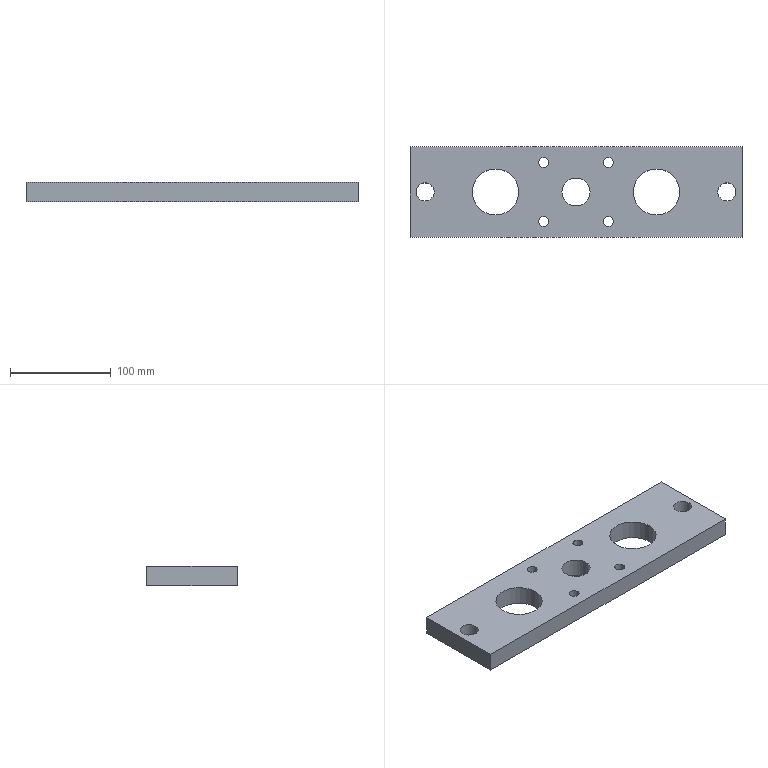Part | NX | features solid 2 | 1 solid | 15 faces | box 330 x 90 x 19 mm | volume 473960 mm3 | cylinder 9 | plane 6 | commonest cylinder face diameters 9.874 x4 18 x2 46 x2 28 x1
STEP:
#1=CARTESIAN_POINT('',(-165.,-15.,-105.));
#2=VERTEX_POINT('',#1);
#3=CARTESIAN_POINT('',(165.,-15.,-105.));
#4=VERTEX_POINT('',#3);
#5=CARTESIAN_POINT('',(-165.,-15.,-105.));
#6=DIRECTION('',(1.,0.,0.));
#7=VECTOR('',#6,1000.);
#8=LINE('',#5,#7);
#9=EDGE_CURVE('',#2,#4,#8,.T.);
#10=ORIENTED_EDGE('',*,*,#9,.F.);
#11=CARTESIAN_POINT('',(-165.,-15.,-86.));
#12=VERTEX_POINT('',#11);
#13=CARTESIAN_POINT('',(-165.,-15.,-86.));
#14=DIRECTION('',(0.,0.,-1.));
#15=VECTOR('',#14,1000.);
#16=LINE('',#13,#15);
#17=EDGE_CURVE('',#12,#2,#16,.T.);
#18=ORIENTED_EDGE('',*,*,#17,.F.);
#19=CARTESIAN_POINT('',(165.,-15.,-86.));
#20=VERTEX_POINT('',#19);
#21=CARTESIAN_POINT('',(-165.,-15.,-86.));
#22=DIRECTION('',(1.,0.,0.));
#23=VECTOR('',#22,1000.);
#24=LINE('',#21,#23);
#25=EDGE_CURVE('',#12,#20,#24,.T.);
#26=ORIENTED_EDGE('',*,*,#25,.T.);
#27=CARTESIAN_POINT('',(165.,-15.,-86.));
#28=DIRECTION('',(0.,0.,-1.));
#29=VECTOR('',#28,1000.);
#30=LINE('',#27,#29);
#31=EDGE_CURVE('',#20,#4,#30,.T.);
#32=ORIENTED_EDGE('',*,*,#31,.T.);
#33=EDGE_LOOP('',(#10,#18,#26,#32));
#34=FACE_BOUND('',#33,.T.);
#35=CARTESIAN_POINT('',(-165.,-15.,-86.));
#36=DIRECTION('',(0.,1.,0.));
#37=DIRECTION('',(0.,0.,1.));
#38=AXIS2_PLACEMENT_3D('',#35,#36,#37);
#39=PLANE('',#38);
#40=ADVANCED_FACE('',(#34),#39,.T.);
#41=CARTESIAN_POINT('',(-165.,-105.,-105.));
#42=VERTEX_POINT('',#41);
#43=CARTESIAN_POINT('',(-165.,-60.,-105.));
#44=DIRECTION('',(0.,-1.,0.));
#45=VECTOR('',#44,1000.);
#46=LINE('',#43,#45);
#47=EDGE_CURVE('',#2,#42,#46,.T.);
#48=ORIENTED_EDGE('',*,*,#47,.T.);
#49=CARTESIAN_POINT('',(-165.,-105.,-86.));
#50=VERTEX_POINT('',#49);
#51=CARTESIAN_POINT('',(-165.,-105.,-86.));
#52=DIRECTION('',(0.,0.,-1.));
#53=VECTOR('',#52,1000.);
#54=LINE('',#51,#53);
#55=EDGE_CURVE('',#50,#42,#54,.T.);
#56=ORIENTED_EDGE('',*,*,#55,.F.);
#57=CARTESIAN_POINT('',(-165.,-60.,-86.));
#58=DIRECTION('',(0.,-1.,0.));
#59=VECTOR('',#58,1000.);
#60=LINE('',#57,#59);
#61=EDGE_CURVE('',#12,#50,#60,.T.);
#62=ORIENTED_EDGE('',*,*,#61,.F.);
#63=ORIENTED_EDGE('',*,*,#17,.T.);
#64=EDGE_LOOP('',(#48,#56,#62,#63));
#65=FACE_BOUND('',#64,.T.);
#66=CARTESIAN_POINT('',(-165.,-60.,-86.));
#67=DIRECTION('',(1.,0.,0.));
#68=DIRECTION('',(0.,0.,-1.));
#69=AXIS2_PLACEMENT_3D('',#66,#67,#68);
#70=PLANE('',#69);
#71=ADVANCED_FACE('',(#65),#70,.F.);
#72=CARTESIAN_POINT('',(165.,-105.,-105.));
#73=VERTEX_POINT('',#72);
#74=CARTESIAN_POINT('',(165.,-105.,-105.));
#75=DIRECTION('',(-1.,0.,0.));
#76=VECTOR('',#75,1000.);
#77=LINE('',#74,#76);
#78=EDGE_CURVE('',#73,#42,#77,.T.);
#79=ORIENTED_EDGE('',*,*,#78,.F.);
#80=CARTESIAN_POINT('',(165.,-105.,-86.));
#81=VERTEX_POINT('',#80);
#82=CARTESIAN_POINT('',(165.,-105.,-86.));
#83=DIRECTION('',(0.,0.,-1.));
#84=VECTOR('',#83,1000.);
#85=LINE('',#82,#84);
#86=EDGE_CURVE('',#81,#73,#85,.T.);
#87=ORIENTED_EDGE('',*,*,#86,.F.);
#88=CARTESIAN_POINT('',(165.,-105.,-86.));
#89=DIRECTION('',(-1.,0.,0.));
#90=VECTOR('',#89,1000.);
#91=LINE('',#88,#90);
#92=EDGE_CURVE('',#81,#50,#91,.T.);
#93=ORIENTED_EDGE('',*,*,#92,.T.);
#94=ORIENTED_EDGE('',*,*,#55,.T.);
#95=EDGE_LOOP('',(#79,#87,#93,#94));
#96=FACE_BOUND('',#95,.T.);
#97=CARTESIAN_POINT('',(165.,-105.,-86.));
#98=DIRECTION('',(0.,-1.,0.));
#99=DIRECTION('',(1.,0.,0.));
#100=AXIS2_PLACEMENT_3D('',#97,#98,#99);
#101=PLANE('',#100);
#102=ADVANCED_FACE('',(#96),#101,.T.);
#103=CARTESIAN_POINT('',(-37.06,-30.594,-86.));
#104=VERTEX_POINT('',#103);
#105=CARTESIAN_POINT('',(-32.124,-30.594,-86.));
#106=DIRECTION('',(0.,0.,1.));
#107=DIRECTION('',(-1.,0.,0.));
#108=AXIS2_PLACEMENT_3D('',#105,#106,#107);
#109=CIRCLE('',#108,4.937);
#110=EDGE_CURVE('',#104,#104,#109,.T.);
#111=ORIENTED_EDGE('',*,*,#110,.T.);
#112=EDGE_LOOP('',(#111));
#113=FACE_BOUND('',#112,.T.);
#114=CARTESIAN_POINT('',(-37.06,-30.594,-105.));
#115=VERTEX_POINT('',#114);
#116=CARTESIAN_POINT('',(-32.124,-30.594,-105.));
#117=DIRECTION('',(0.,0.,1.));
#118=DIRECTION('',(-1.,0.,0.));
#119=AXIS2_PLACEMENT_3D('',#116,#117,#118);
#120=CIRCLE('',#119,4.937);
#121=EDGE_CURVE('',#115,#115,#120,.T.);
#122=ORIENTED_EDGE('',*,*,#121,.F.);
#123=EDGE_LOOP('',(#122));
#124=FACE_BOUND('',#123,.T.);
#125=CARTESIAN_POINT('',(-32.124,-30.594,-86.));
#126=DIRECTION('',(0.,0.,-1.));
#127=DIRECTION('',(-1.,0.,0.));
#128=AXIS2_PLACEMENT_3D('',#125,#126,#127);
#129=CYLINDRICAL_SURFACE('',#128,4.937);
#130=ADVANCED_FACE('',(#113,#124),#129,.F.);
#131=CARTESIAN_POINT('',(57.,-60.,-86.));
#132=VERTEX_POINT('',#131);
#133=CARTESIAN_POINT('',(80.,-60.,-86.));
#134=DIRECTION('',(0.,0.,-1.));
#135=DIRECTION('',(-1.,0.,0.));
#136=AXIS2_PLACEMENT_3D('',#133,#134,#135);
#137=CIRCLE('',#136,23.);
#138=EDGE_CURVE('',#132,#132,#137,.T.);
#139=ORIENTED_EDGE('',*,*,#138,.F.);
#140=EDGE_LOOP('',(#139));
#141=FACE_BOUND('',#140,.T.);
#142=CARTESIAN_POINT('',(57.,-60.,-105.));
#143=VERTEX_POINT('',#142);
#144=CARTESIAN_POINT('',(80.,-60.,-105.));
#145=DIRECTION('',(0.,0.,-1.));
#146=DIRECTION('',(-1.,0.,0.));
#147=AXIS2_PLACEMENT_3D('',#144,#145,#146);
#148=CIRCLE('',#147,23.);
#149=EDGE_CURVE('',#143,#143,#148,.T.);
#150=ORIENTED_EDGE('',*,*,#149,.T.);
#151=EDGE_LOOP('',(#150));
#152=FACE_BOUND('',#151,.T.);
#153=CARTESIAN_POINT('',(80.,-60.,-86.));
#154=DIRECTION('',(0.,0.,-1.));
#155=DIRECTION('',(-1.,0.,0.));
#156=AXIS2_PLACEMENT_3D('',#153,#154,#155);
#157=CYLINDRICAL_SURFACE('',#156,23.);
#158=ADVANCED_FACE('',(#141,#152),#157,.F.);
#159=CARTESIAN_POINT('',(-141.,-60.,-86.));
#160=VERTEX_POINT('',#159);
#161=CARTESIAN_POINT('',(-150.,-60.,-86.));
#162=DIRECTION('',(0.,0.,1.));
#163=DIRECTION('',(1.,0.,0.));
#164=AXIS2_PLACEMENT_3D('',#161,#162,#163);
#165=CIRCLE('',#164,9.);
#166=EDGE_CURVE('',#160,#160,#165,.T.);
#167=ORIENTED_EDGE('',*,*,#166,.T.);
#168=EDGE_LOOP('',(#167));
#169=FACE_BOUND('',#168,.T.);
#170=CARTESIAN_POINT('',(-141.,-60.,-105.));
#171=VERTEX_POINT('',#170);
#172=CARTESIAN_POINT('',(-150.,-60.,-105.));
#173=DIRECTION('',(0.,0.,1.));
#174=DIRECTION('',(1.,0.,0.));
#175=AXIS2_PLACEMENT_3D('',#172,#173,#174);
#176=CIRCLE('',#175,9.);
#177=EDGE_CURVE('',#171,#171,#176,.T.);
#178=ORIENTED_EDGE('',*,*,#177,.F.);
#179=EDGE_LOOP('',(#178));
#180=FACE_BOUND('',#179,.T.);
#181=CARTESIAN_POINT('',(-150.,-60.,-86.));
#182=DIRECTION('',(0.,0.,-1.));
#183=DIRECTION('',(-1.,0.,0.));
#184=AXIS2_PLACEMENT_3D('',#181,#182,#183);
#185=CYLINDRICAL_SURFACE('',#184,9.);
#186=ADVANCED_FACE('',(#169,#180),#185,.F.);
#187=CARTESIAN_POINT('',(165.,-60.,-105.));
#188=DIRECTION('',(0.,-1.,0.));
#189=VECTOR('',#188,1000.);
#190=LINE('',#187,#189);
#191=EDGE_CURVE('',#4,#73,#190,.T.);
#192=ORIENTED_EDGE('',*,*,#191,.F.);
#193=ORIENTED_EDGE('',*,*,#31,.F.);
#194=CARTESIAN_POINT('',(165.,-60.,-86.));
#195=DIRECTION('',(0.,-1.,0.));
#196=VECTOR('',#195,1000.);
#197=LINE('',#194,#196);
#198=EDGE_CURVE('',#20,#81,#197,.T.);
#199=ORIENTED_EDGE('',*,*,#198,.T.);
#200=ORIENTED_EDGE('',*,*,#86,.T.);
#201=EDGE_LOOP('',(#192,#193,#199,#200));
#202=FACE_BOUND('',#201,.T.);
#203=CARTESIAN_POINT('',(165.,-60.,-86.));
#204=DIRECTION('',(1.,0.,0.));
#205=DIRECTION('',(0.,0.,-1.));
#206=AXIS2_PLACEMENT_3D('',#203,#204,#205);
#207=PLANE('',#206);
#208=ADVANCED_FACE('',(#202),#207,.T.);
#209=CARTESIAN_POINT('',(141.,-60.,-86.));
#210=VERTEX_POINT('',#209);
#211=CARTESIAN_POINT('',(150.,-60.,-86.));
#212=DIRECTION('',(0.,0.,-1.));
#213=DIRECTION('',(-1.,0.,0.));
#214=AXIS2_PLACEMENT_3D('',#211,#212,#213);
#215=CIRCLE('',#214,9.);
#216=EDGE_CURVE('',#210,#210,#215,.T.);
#217=ORIENTED_EDGE('',*,*,#216,.F.);
#218=EDGE_LOOP('',(#217));
#219=FACE_BOUND('',#218,.T.);
#220=CARTESIAN_POINT('',(141.,-60.,-105.));
#221=VERTEX_POINT('',#220);
#222=CARTESIAN_POINT('',(150.,-60.,-105.));
#223=DIRECTION('',(0.,0.,-1.));
#224=DIRECTION('',(-1.,0.,0.));
#225=AXIS2_PLACEMENT_3D('',#222,#223,#224);
#226=CIRCLE('',#225,9.);
#227=EDGE_CURVE('',#221,#221,#226,.T.);
#228=ORIENTED_EDGE('',*,*,#227,.T.);
#229=EDGE_LOOP('',(#228));
#230=FACE_BOUND('',#229,.T.);
#231=CARTESIAN_POINT('',(150.,-60.,-86.));
#232=DIRECTION('',(0.,0.,-1.));
#233=DIRECTION('',(-1.,0.,0.));
#234=AXIS2_PLACEMENT_3D('',#231,#232,#233);
#235=CYLINDRICAL_SURFACE('',#234,9.);
#236=ADVANCED_FACE('',(#219,#230),#235,.F.);
#237=CARTESIAN_POINT('',(-57.,-60.,-86.));
#238=VERTEX_POINT('',#237);
#239=CARTESIAN_POINT('',(-80.,-60.,-86.));
#240=DIRECTION('',(0.,0.,1.));
#241=DIRECTION('',(1.,0.,0.));
#242=AXIS2_PLACEMENT_3D('',#239,#240,#241);
#243=CIRCLE('',#242,23.);
#244=EDGE_CURVE('',#238,#238,#243,.T.);
#245=ORIENTED_EDGE('',*,*,#244,.T.);
#246=EDGE_LOOP('',(#245));
#247=FACE_BOUND('',#246,.T.);
#248=CARTESIAN_POINT('',(-57.,-60.,-105.));
#249=VERTEX_POINT('',#248);
#250=CARTESIAN_POINT('',(-80.,-60.,-105.));
#251=DIRECTION('',(0.,0.,1.));
#252=DIRECTION('',(1.,0.,0.));
#253=AXIS2_PLACEMENT_3D('',#250,#251,#252);
#254=CIRCLE('',#253,23.);
#255=EDGE_CURVE('',#249,#249,#254,.T.);
#256=ORIENTED_EDGE('',*,*,#255,.F.);
#257=EDGE_LOOP('',(#256));
#258=FACE_BOUND('',#257,.T.);
#259=CARTESIAN_POINT('',(-80.,-60.,-86.));
#260=DIRECTION('',(0.,0.,-1.));
#261=DIRECTION('',(-1.,0.,0.));
#262=AXIS2_PLACEMENT_3D('',#259,#260,#261);
#263=CYLINDRICAL_SURFACE('',#262,23.);
#264=ADVANCED_FACE('',(#247,#258),#263,.F.);
#265=CARTESIAN_POINT('',(37.06,-30.594,-86.));
#266=VERTEX_POINT('',#265);
#267=CARTESIAN_POINT('',(32.124,-30.594,-86.));
#268=DIRECTION('',(0.,0.,-1.));
#269=DIRECTION('',(1.,0.,0.));
#270=AXIS2_PLACEMENT_3D('',#267,#268,#269);
#271=CIRCLE('',#270,4.937);
#272=EDGE_CURVE('',#266,#266,#271,.T.);
#273=ORIENTED_EDGE('',*,*,#272,.F.);
#274=EDGE_LOOP('',(#273));
#275=FACE_BOUND('',#274,.T.);
#276=CARTESIAN_POINT('',(37.06,-30.594,-105.));
#277=VERTEX_POINT('',#276);
#278=CARTESIAN_POINT('',(32.124,-30.594,-105.));
#279=DIRECTION('',(0.,0.,-1.));
#280=DIRECTION('',(1.,0.,0.));
#281=AXIS2_PLACEMENT_3D('',#278,#279,#280);
#282=CIRCLE('',#281,4.937);
#283=EDGE_CURVE('',#277,#277,#282,.T.);
#284=ORIENTED_EDGE('',*,*,#283,.T.);
#285=EDGE_LOOP('',(#284));
#286=FACE_BOUND('',#285,.T.);
#287=CARTESIAN_POINT('',(32.124,-30.594,-86.));
#288=DIRECTION('',(0.,0.,-1.));
#289=DIRECTION('',(-1.,0.,0.));
#290=AXIS2_PLACEMENT_3D('',#287,#288,#289);
#291=CYLINDRICAL_SURFACE('',#290,4.937);
#292=ADVANCED_FACE('',(#275,#286),#291,.F.);
#293=CARTESIAN_POINT('',(37.06,-89.406,-86.));
#294=VERTEX_POINT('',#293);
#295=CARTESIAN_POINT('',(32.124,-89.406,-86.));
#296=DIRECTION('',(0.,0.,1.));
#297=DIRECTION('',(1.,0.,0.));
#298=AXIS2_PLACEMENT_3D('',#295,#296,#297);
#299=CIRCLE('',#298,4.937);
#300=EDGE_CURVE('',#294,#294,#299,.T.);
#301=ORIENTED_EDGE('',*,*,#300,.T.);
#302=EDGE_LOOP('',(#301));
#303=FACE_BOUND('',#302,.T.);
#304=CARTESIAN_POINT('',(37.06,-89.406,-105.));
#305=VERTEX_POINT('',#304);
#306=CARTESIAN_POINT('',(32.124,-89.406,-105.));
#307=DIRECTION('',(0.,0.,1.));
#308=DIRECTION('',(1.,0.,0.));
#309=AXIS2_PLACEMENT_3D('',#306,#307,#308);
#310=CIRCLE('',#309,4.937);
#311=EDGE_CURVE('',#305,#305,#310,.T.);
#312=ORIENTED_EDGE('',*,*,#311,.F.);
#313=EDGE_LOOP('',(#312));
#314=FACE_BOUND('',#313,.T.);
#315=CARTESIAN_POINT('',(32.124,-89.406,-86.));
#316=DIRECTION('',(0.,0.,-1.));
#317=DIRECTION('',(-1.,0.,0.));
#318=AXIS2_PLACEMENT_3D('',#315,#316,#317);
#319=CYLINDRICAL_SURFACE('',#318,4.937);
#320=ADVANCED_FACE('',(#303,#314),#319,.F.);
#321=CARTESIAN_POINT('',(14.,-60.,-86.));
#322=VERTEX_POINT('',#321);
#323=CARTESIAN_POINT('',(0.,-60.,-86.));
#324=DIRECTION('',(0.,0.,1.));
#325=DIRECTION('',(1.,0.,0.));
#326=AXIS2_PLACEMENT_3D('',#323,#324,#325);
#327=CIRCLE('',#326,14.);
#328=EDGE_CURVE('',#322,#322,#327,.T.);
#329=ORIENTED_EDGE('',*,*,#328,.T.);
#330=EDGE_LOOP('',(#329));
#331=FACE_BOUND('',#330,.T.);
#332=CARTESIAN_POINT('',(14.,-60.,-105.));
#333=VERTEX_POINT('',#332);
#334=CARTESIAN_POINT('',(0.,-60.,-105.));
#335=DIRECTION('',(0.,0.,1.));
#336=DIRECTION('',(1.,0.,0.));
#337=AXIS2_PLACEMENT_3D('',#334,#335,#336);
#338=CIRCLE('',#337,14.);
#339=EDGE_CURVE('',#333,#333,#338,.T.);
#340=ORIENTED_EDGE('',*,*,#339,.F.);
#341=EDGE_LOOP('',(#340));
#342=FACE_BOUND('',#341,.T.);
#343=CARTESIAN_POINT('',(0.,-60.,-86.));
#344=DIRECTION('',(0.,0.,-1.));
#345=DIRECTION('',(-1.,0.,0.));
#346=AXIS2_PLACEMENT_3D('',#343,#344,#345);
#347=CYLINDRICAL_SURFACE('',#346,14.);
#348=ADVANCED_FACE('',(#331,#342),#347,.F.);
#349=CARTESIAN_POINT('',(-37.06,-89.406,-86.));
#350=VERTEX_POINT('',#349);
#351=CARTESIAN_POINT('',(-32.124,-89.406,-86.));
#352=DIRECTION('',(0.,0.,-1.));
#353=DIRECTION('',(-1.,0.,0.));
#354=AXIS2_PLACEMENT_3D('',#351,#352,#353);
#355=CIRCLE('',#354,4.937);
#356=EDGE_CURVE('',#350,#350,#355,.T.);
#357=ORIENTED_EDGE('',*,*,#356,.F.);
#358=EDGE_LOOP('',(#357));
#359=FACE_BOUND('',#358,.T.);
#360=CARTESIAN_POINT('',(-37.06,-89.406,-105.));
#361=VERTEX_POINT('',#360);
#362=CARTESIAN_POINT('',(-32.124,-89.406,-105.));
#363=DIRECTION('',(0.,0.,-1.));
#364=DIRECTION('',(-1.,0.,0.));
#365=AXIS2_PLACEMENT_3D('',#362,#363,#364);
#366=CIRCLE('',#365,4.937);
#367=EDGE_CURVE('',#361,#361,#366,.T.);
#368=ORIENTED_EDGE('',*,*,#367,.T.);
#369=EDGE_LOOP('',(#368));
#370=FACE_BOUND('',#369,.T.);
#371=CARTESIAN_POINT('',(-32.124,-89.406,-86.));
#372=DIRECTION('',(0.,0.,-1.));
#373=DIRECTION('',(-1.,0.,0.));
#374=AXIS2_PLACEMENT_3D('',#371,#372,#373);
#375=CYLINDRICAL_SURFACE('',#374,4.937);
#376=ADVANCED_FACE('',(#359,#370),#375,.F.);
#377=ORIENTED_EDGE('',*,*,#328,.F.);
#378=EDGE_LOOP('',(#377));
#379=FACE_BOUND('',#378,.T.);
#380=ORIENTED_EDGE('',*,*,#300,.F.);
#381=EDGE_LOOP('',(#380));
#382=FACE_BOUND('',#381,.T.);
#383=ORIENTED_EDGE('',*,*,#272,.T.);
#384=EDGE_LOOP('',(#383));
#385=FACE_BOUND('',#384,.T.);
#386=ORIENTED_EDGE('',*,*,#244,.F.);
#387=EDGE_LOOP('',(#386));
#388=FACE_BOUND('',#387,.T.);
#389=ORIENTED_EDGE('',*,*,#216,.T.);
#390=EDGE_LOOP('',(#389));
#391=FACE_BOUND('',#390,.T.);
#392=ORIENTED_EDGE('',*,*,#198,.F.);
#393=ORIENTED_EDGE('',*,*,#25,.F.);
#394=ORIENTED_EDGE('',*,*,#61,.T.);
#395=ORIENTED_EDGE('',*,*,#92,.F.);
#396=EDGE_LOOP('',(#392,#393,#394,#395));
#397=FACE_BOUND('',#396,.T.);
#398=ORIENTED_EDGE('',*,*,#166,.F.);
#399=EDGE_LOOP('',(#398));
#400=FACE_BOUND('',#399,.T.);
#401=ORIENTED_EDGE('',*,*,#138,.T.);
#402=EDGE_LOOP('',(#401));
#403=FACE_BOUND('',#402,.T.);
#404=ORIENTED_EDGE('',*,*,#110,.F.);
#405=EDGE_LOOP('',(#404));
#406=FACE_BOUND('',#405,.T.);
#407=ORIENTED_EDGE('',*,*,#356,.T.);
#408=EDGE_LOOP('',(#407));
#409=FACE_BOUND('',#408,.T.);
#410=CARTESIAN_POINT('',(165.,-105.,-86.));
#411=DIRECTION('',(0.,0.,-1.));
#412=DIRECTION('',(-1.,0.,0.));
#413=AXIS2_PLACEMENT_3D('',#410,#411,#412);
#414=PLANE('',#413);
#415=ADVANCED_FACE('',(#379,#382,#385,#388,#391,#397,#400,#403,#406,#409),#414,.F.);
#416=ORIENTED_EDGE('',*,*,#339,.T.);
#417=EDGE_LOOP('',(#416));
#418=FACE_BOUND('',#417,.T.);
#419=ORIENTED_EDGE('',*,*,#311,.T.);
#420=EDGE_LOOP('',(#419));
#421=FACE_BOUND('',#420,.T.);
#422=ORIENTED_EDGE('',*,*,#283,.F.);
#423=EDGE_LOOP('',(#422));
#424=FACE_BOUND('',#423,.T.);
#425=ORIENTED_EDGE('',*,*,#255,.T.);
#426=EDGE_LOOP('',(#425));
#427=FACE_BOUND('',#426,.T.);
#428=ORIENTED_EDGE('',*,*,#227,.F.);
#429=EDGE_LOOP('',(#428));
#430=FACE_BOUND('',#429,.T.);
#431=ORIENTED_EDGE('',*,*,#9,.T.);
#432=ORIENTED_EDGE('',*,*,#191,.T.);
#433=ORIENTED_EDGE('',*,*,#78,.T.);
#434=ORIENTED_EDGE('',*,*,#47,.F.);
#435=EDGE_LOOP('',(#431,#432,#433,#434));
#436=FACE_BOUND('',#435,.T.);
#437=ORIENTED_EDGE('',*,*,#177,.T.);
#438=EDGE_LOOP('',(#437));
#439=FACE_BOUND('',#438,.T.);
#440=ORIENTED_EDGE('',*,*,#149,.F.);
#441=EDGE_LOOP('',(#440));
#442=FACE_BOUND('',#441,.T.);
#443=ORIENTED_EDGE('',*,*,#121,.T.);
#444=EDGE_LOOP('',(#443));
#445=FACE_BOUND('',#444,.T.);
#446=ORIENTED_EDGE('',*,*,#367,.F.);
#447=EDGE_LOOP('',(#446));
#448=FACE_BOUND('',#447,.T.);
#449=CARTESIAN_POINT('',(165.,-105.,-105.));
#450=DIRECTION('',(0.,0.,-1.));
#451=DIRECTION('',(-1.,0.,0.));
#452=AXIS2_PLACEMENT_3D('',#449,#450,#451);
#453=PLANE('',#452);
#454=ADVANCED_FACE('',(#418,#421,#424,#427,#430,#436,#439,#442,#445,#448),#453,.T.);
#455=CLOSED_SHELL('',(#40,#71,#102,#130,#158,#186,#208,#236,#264,#292,#320,#348,#376,#415,#454));
#456=MANIFOLD_SOLID_BREP('',#455);
#457=(LENGTH_UNIT()NAMED_UNIT(*)SI_UNIT(.MILLI.,.METRE.));
#458=UNCERTAINTY_MEASURE_WITH_UNIT(LENGTH_MEASURE(0.00001),#457,'','');
#459=(NAMED_UNIT(*)PLANE_ANGLE_UNIT()SI_UNIT($,.RADIAN.));
#460=(NAMED_UNIT(*)SI_UNIT($,.STERADIAN.)SOLID_ANGLE_UNIT());
#461=(GEOMETRIC_REPRESENTATION_CONTEXT(3)GLOBAL_UNCERTAINTY_ASSIGNED_CONTEXT((#458))GLOBAL_UNIT_ASSIGNED_CONTEXT((#457,#459,#460))REPRESENTATION_CONTEXT('',''));
#462=ADVANCED_BREP_SHAPE_REPRESENTATION('',(#456),#461);